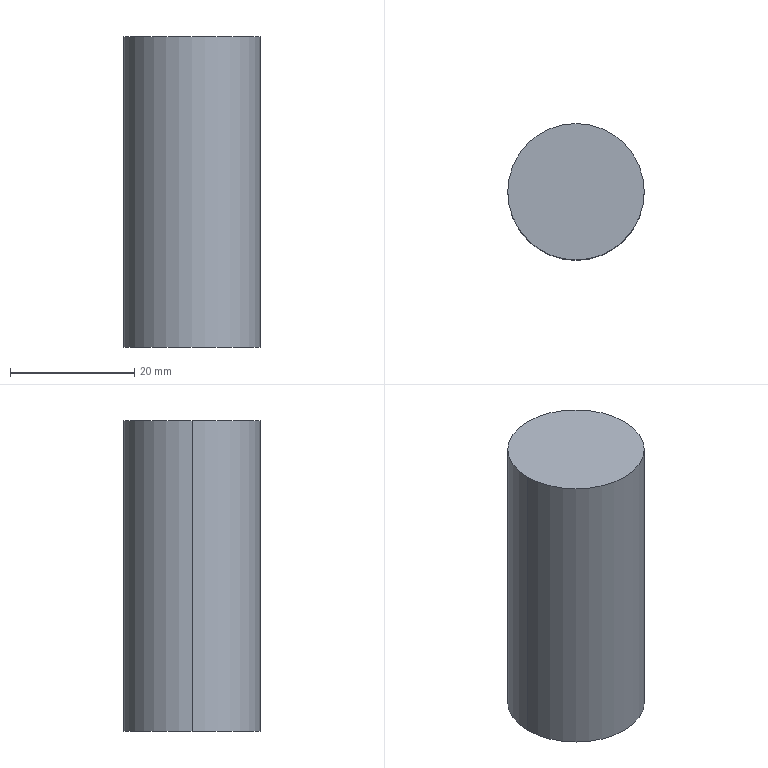Part | STEP file | copper tube 36 | 1 solid | 4 faces | box 22 x 22 x 50 mm | volume 19007 mm3 | cylinder 2 | plane 2 | commonest cylinder face diameters 22 x2
STEP:
#1=CARTESIAN_POINT('',(0.,0.,0.));
#2=DIRECTION('',(0.,0.,1.));
#3=DIRECTION('',(1.,0.,0.));
#4=AXIS2_PLACEMENT_3D('',#1,#2,#3);
#5=CARTESIAN_POINT('',(11.,0.,50.));
#6=VERTEX_POINT('',#5);
#7=CARTESIAN_POINT('',(-11.,0.,50.));
#8=VERTEX_POINT('',#7);
#9=CARTESIAN_POINT('',(0.,0.,50.));
#10=DIRECTION('',(0.,0.,1.));
#11=DIRECTION('',(1.,0.,0.));
#12=AXIS2_PLACEMENT_3D('',#9,#10,#11);
#13=CIRCLE('',#12,11.);
#14=CARTESIAN_POINT('',(0.,0.,50.));
#15=DIRECTION('',(0.,0.,-1.));
#16=DIRECTION('',(-1.,0.,0.));
#17=AXIS2_PLACEMENT_3D('',#14,#15,#16);
#18=CYLINDRICAL_SURFACE('',#17,11.);
#19=CARTESIAN_POINT('',(3.142,0.));
#20=DIRECTION('',(-1.,0.));
#21=VECTOR('',#20,1.);
#22=LINE('',#19,#21);
#23=(GEOMETRIC_REPRESENTATION_CONTEXT(2)PARAMETRIC_REPRESENTATION_CONTEXT()REPRESENTATION_CONTEXT('',''));
#24=DEFINITIONAL_REPRESENTATION('',(#22),#23);
#25=PCURVE('',#18,#24);
#26=CARTESIAN_POINT('',(0.,0.,50.));
#27=DIRECTION('',(0.,0.,1.));
#28=DIRECTION('',(1.,0.,0.));
#29=AXIS2_PLACEMENT_3D('',#26,#27,#28);
#30=PLANE('',#29);
#31=CARTESIAN_POINT('',(0.,0.));
#32=DIRECTION('',(1.,0.));
#33=AXIS2_PLACEMENT_2D('',#31,#32);
#34=CIRCLE('',#33,11.);
#35=(GEOMETRIC_REPRESENTATION_CONTEXT(2)PARAMETRIC_REPRESENTATION_CONTEXT()REPRESENTATION_CONTEXT('',''));
#36=DEFINITIONAL_REPRESENTATION('',(#34),#35);
#37=PCURVE('',#30,#36);
#38=SURFACE_CURVE('',#13,(#25,#37),.PCURVE_S1.);
#39=EDGE_CURVE('',#6,#8,#38,.T.);
#40=ORIENTED_EDGE('',*,*,#39,.F.);
#41=CARTESIAN_POINT('',(11.,0.,0.));
#42=VERTEX_POINT('',#41);
#43=CARTESIAN_POINT('',(11.,0.,50.));
#44=DIRECTION('',(0.,0.,-1.));
#45=VECTOR('',#44,1.);
#46=LINE('',#43,#45);
#47=CARTESIAN_POINT('',(3.142,0.));
#48=DIRECTION('',(0.,1.));
#49=VECTOR('',#48,1.);
#50=LINE('',#47,#49);
#51=(GEOMETRIC_REPRESENTATION_CONTEXT(2)PARAMETRIC_REPRESENTATION_CONTEXT()REPRESENTATION_CONTEXT('',''));
#52=DEFINITIONAL_REPRESENTATION('',(#50),#51);
#53=PCURVE('',#18,#52);
#54=CARTESIAN_POINT('',(0.,0.,50.));
#55=DIRECTION('',(0.,0.,-1.));
#56=DIRECTION('',(-1.,0.,0.));
#57=AXIS2_PLACEMENT_3D('',#54,#55,#56);
#58=CYLINDRICAL_SURFACE('',#57,11.);
#59=CARTESIAN_POINT('',(3.142,0.));
#60=DIRECTION('',(0.,1.));
#61=VECTOR('',#60,1.);
#62=LINE('',#59,#61);
#63=(GEOMETRIC_REPRESENTATION_CONTEXT(2)PARAMETRIC_REPRESENTATION_CONTEXT()REPRESENTATION_CONTEXT('',''));
#64=DEFINITIONAL_REPRESENTATION('',(#62),#63);
#65=PCURVE('',#58,#64);
#66=SURFACE_CURVE('',#46,(#53,#65),.PCURVE_S1.);
#67=EDGE_CURVE('',#6,#42,#66,.T.);
#68=ORIENTED_EDGE('',*,*,#67,.T.);
#69=CARTESIAN_POINT('',(-11.,0.,0.));
#70=VERTEX_POINT('',#69);
#71=CARTESIAN_POINT('',(0.,0.,0.));
#72=DIRECTION('',(0.,0.,1.));
#73=DIRECTION('',(1.,0.,0.));
#74=AXIS2_PLACEMENT_3D('',#71,#72,#73);
#75=CIRCLE('',#74,11.);
#76=CARTESIAN_POINT('',(3.142,50.));
#77=DIRECTION('',(-1.,0.));
#78=VECTOR('',#77,1.);
#79=LINE('',#76,#78);
#80=(GEOMETRIC_REPRESENTATION_CONTEXT(2)PARAMETRIC_REPRESENTATION_CONTEXT()REPRESENTATION_CONTEXT('',''));
#81=DEFINITIONAL_REPRESENTATION('',(#79),#80);
#82=PCURVE('',#18,#81);
#83=CARTESIAN_POINT('',(0.,0.,0.));
#84=DIRECTION('',(0.,0.,1.));
#85=DIRECTION('',(1.,0.,0.));
#86=AXIS2_PLACEMENT_3D('',#83,#84,#85);
#87=PLANE('',#86);
#88=CARTESIAN_POINT('',(0.,0.));
#89=DIRECTION('',(1.,0.));
#90=AXIS2_PLACEMENT_2D('',#88,#89);
#91=CIRCLE('',#90,11.);
#92=(GEOMETRIC_REPRESENTATION_CONTEXT(2)PARAMETRIC_REPRESENTATION_CONTEXT()REPRESENTATION_CONTEXT('',''));
#93=DEFINITIONAL_REPRESENTATION('',(#91),#92);
#94=PCURVE('',#87,#93);
#95=SURFACE_CURVE('',#75,(#82,#94),.PCURVE_S1.);
#96=EDGE_CURVE('',#42,#70,#95,.T.);
#97=ORIENTED_EDGE('',*,*,#96,.T.);
#98=CARTESIAN_POINT('',(-11.,0.,50.));
#99=DIRECTION('',(0.,0.,-1.));
#100=VECTOR('',#99,1.);
#101=LINE('',#98,#100);
#102=CARTESIAN_POINT('',(0.,0.));
#103=DIRECTION('',(0.,1.));
#104=VECTOR('',#103,1.);
#105=LINE('',#102,#104);
#106=(GEOMETRIC_REPRESENTATION_CONTEXT(2)PARAMETRIC_REPRESENTATION_CONTEXT()REPRESENTATION_CONTEXT('',''));
#107=DEFINITIONAL_REPRESENTATION('',(#105),#106);
#108=PCURVE('',#18,#107);
#109=CARTESIAN_POINT('',(6.283,0.));
#110=DIRECTION('',(0.,1.));
#111=VECTOR('',#110,1.);
#112=LINE('',#109,#111);
#113=(GEOMETRIC_REPRESENTATION_CONTEXT(2)PARAMETRIC_REPRESENTATION_CONTEXT()REPRESENTATION_CONTEXT('',''));
#114=DEFINITIONAL_REPRESENTATION('',(#112),#113);
#115=PCURVE('',#58,#114);
#116=SURFACE_CURVE('',#101,(#108,#115),.PCURVE_S1.);
#117=EDGE_CURVE('',#8,#70,#116,.T.);
#118=ORIENTED_EDGE('',*,*,#117,.F.);
#119=EDGE_LOOP('',(#40,#68,#97,#118));
#120=FACE_BOUND('',#119,.T.);
#121=ADVANCED_FACE('',(#120),#18,.T.);
#122=ORIENTED_EDGE('',*,*,#67,.F.);
#123=CARTESIAN_POINT('',(0.,0.,50.));
#124=DIRECTION('',(0.,0.,1.));
#125=DIRECTION('',(1.,0.,0.));
#126=AXIS2_PLACEMENT_3D('',#123,#124,#125);
#127=CIRCLE('',#126,11.);
#128=CARTESIAN_POINT('',(9.425,0.));
#129=DIRECTION('',(-1.,0.));
#130=VECTOR('',#129,1.);
#131=LINE('',#128,#130);
#132=(GEOMETRIC_REPRESENTATION_CONTEXT(2)PARAMETRIC_REPRESENTATION_CONTEXT()REPRESENTATION_CONTEXT('',''));
#133=DEFINITIONAL_REPRESENTATION('',(#131),#132);
#134=PCURVE('',#58,#133);
#135=CARTESIAN_POINT('',(0.,0.));
#136=DIRECTION('',(1.,0.));
#137=AXIS2_PLACEMENT_2D('',#135,#136);
#138=CIRCLE('',#137,11.);
#139=(GEOMETRIC_REPRESENTATION_CONTEXT(2)PARAMETRIC_REPRESENTATION_CONTEXT()REPRESENTATION_CONTEXT('',''));
#140=DEFINITIONAL_REPRESENTATION('',(#138),#139);
#141=PCURVE('',#30,#140);
#142=SURFACE_CURVE('',#127,(#134,#141),.PCURVE_S1.);
#143=EDGE_CURVE('',#8,#6,#142,.T.);
#144=ORIENTED_EDGE('',*,*,#143,.F.);
#145=ORIENTED_EDGE('',*,*,#117,.T.);
#146=CARTESIAN_POINT('',(0.,0.,0.));
#147=DIRECTION('',(0.,0.,1.));
#148=DIRECTION('',(1.,0.,0.));
#149=AXIS2_PLACEMENT_3D('',#146,#147,#148);
#150=CIRCLE('',#149,11.);
#151=CARTESIAN_POINT('',(9.425,50.));
#152=DIRECTION('',(-1.,0.));
#153=VECTOR('',#152,1.);
#154=LINE('',#151,#153);
#155=(GEOMETRIC_REPRESENTATION_CONTEXT(2)PARAMETRIC_REPRESENTATION_CONTEXT()REPRESENTATION_CONTEXT('',''));
#156=DEFINITIONAL_REPRESENTATION('',(#154),#155);
#157=PCURVE('',#58,#156);
#158=CARTESIAN_POINT('',(0.,0.));
#159=DIRECTION('',(1.,0.));
#160=AXIS2_PLACEMENT_2D('',#158,#159);
#161=CIRCLE('',#160,11.);
#162=(GEOMETRIC_REPRESENTATION_CONTEXT(2)PARAMETRIC_REPRESENTATION_CONTEXT()REPRESENTATION_CONTEXT('',''));
#163=DEFINITIONAL_REPRESENTATION('',(#161),#162);
#164=PCURVE('',#87,#163);
#165=SURFACE_CURVE('',#150,(#157,#164),.PCURVE_S1.);
#166=EDGE_CURVE('',#70,#42,#165,.T.);
#167=ORIENTED_EDGE('',*,*,#166,.T.);
#168=EDGE_LOOP('',(#122,#144,#145,#167));
#169=FACE_BOUND('',#168,.T.);
#170=ADVANCED_FACE('',(#169),#58,.T.);
#171=ORIENTED_EDGE('',*,*,#143,.T.);
#172=ORIENTED_EDGE('',*,*,#39,.T.);
#173=EDGE_LOOP('',(#171,#172));
#174=FACE_BOUND('',#173,.T.);
#175=ADVANCED_FACE('',(#174),#30,.T.);
#176=ORIENTED_EDGE('',*,*,#166,.F.);
#177=ORIENTED_EDGE('',*,*,#96,.F.);
#178=EDGE_LOOP('',(#176,#177));
#179=FACE_BOUND('',#178,.T.);
#180=ADVANCED_FACE('',(#179),#87,.F.);
#181=CLOSED_SHELL('',(#121,#170,#175,#180));
#182=MANIFOLD_SOLID_BREP('',#181);
#183=(LENGTH_UNIT()NAMED_UNIT(*)SI_UNIT(.MILLI.,.METRE.));
#184=UNCERTAINTY_MEASURE_WITH_UNIT(LENGTH_MEASURE(0.0000001),#183,'','');
#185=(NAMED_UNIT(*)PLANE_ANGLE_UNIT()SI_UNIT($,.RADIAN.));
#186=(NAMED_UNIT(*)SI_UNIT($,.STERADIAN.)SOLID_ANGLE_UNIT());
#187=(GEOMETRIC_REPRESENTATION_CONTEXT(3)GLOBAL_UNCERTAINTY_ASSIGNED_CONTEXT((#184))GLOBAL_UNIT_ASSIGNED_CONTEXT((#183,#185,#186))REPRESENTATION_CONTEXT('',''));
#188=ADVANCED_BREP_SHAPE_REPRESENTATION('',(#4,#182),#187);